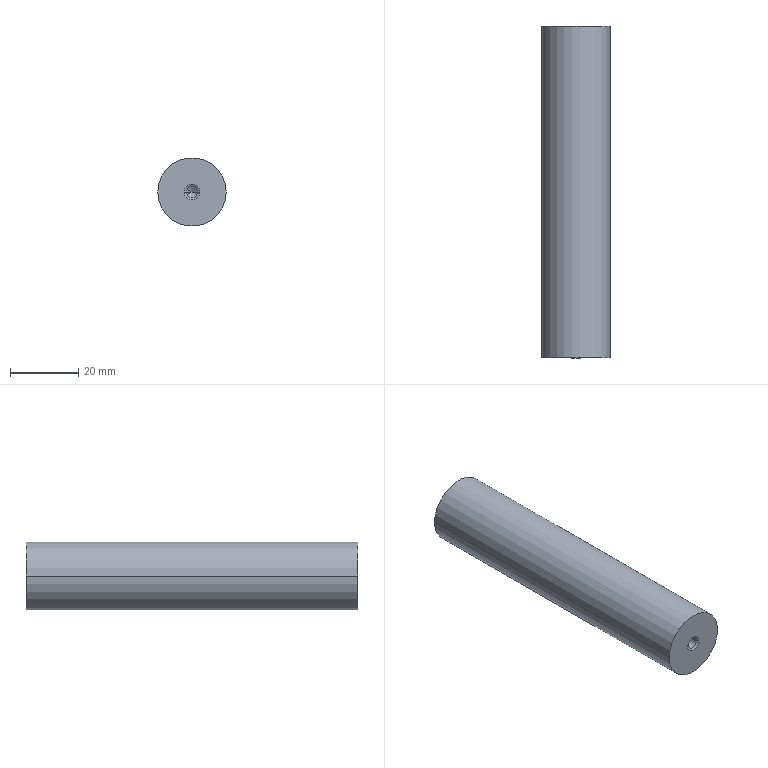Part | NX | 1 solid | 16 faces | box 20 x 97 x 20 mm | volume 30242 mm3 | cone 8 | cylinder 6 | plane 2 | commonest cylinder face diameters 3.3 x4 20 x2
STEP:
#1=CARTESIAN_POINT('',(10.,-28.5,0.));
#2=VERTEX_POINT('',#1);
#3=CARTESIAN_POINT('',(-10.,-28.5,0.));
#4=VERTEX_POINT('',#3);
#5=CARTESIAN_POINT('',(0.,-28.5,0.));
#6=DIRECTION('',(0.,1.,0.));
#7=DIRECTION('',(1.,0.,0.));
#8=AXIS2_PLACEMENT_3D('',#5,#6,#7);
#9=CIRCLE('',#8,10.);
#10=EDGE_CURVE('',#2,#4,#9,.T.);
#11=ORIENTED_EDGE('',*,*,#10,.T.);
#12=CARTESIAN_POINT('',(-10.,68.5,0.));
#13=VERTEX_POINT('',#12);
#14=CARTESIAN_POINT('',(-10.,-44.35,0.));
#15=DIRECTION('',(0.,1.,0.));
#16=VECTOR('',#15,1000.);
#17=LINE('',#14,#16);
#18=EDGE_CURVE('',#13,#4,#17,.F.);
#19=ORIENTED_EDGE('',*,*,#18,.F.);
#20=CARTESIAN_POINT('',(10.,68.5,0.));
#21=VERTEX_POINT('',#20);
#22=CARTESIAN_POINT('',(0.,68.5,0.));
#23=DIRECTION('',(0.,1.,0.));
#24=DIRECTION('',(1.,0.,0.));
#25=AXIS2_PLACEMENT_3D('',#22,#23,#24);
#26=CIRCLE('',#25,10.);
#27=EDGE_CURVE('',#21,#13,#26,.T.);
#28=ORIENTED_EDGE('',*,*,#27,.F.);
#29=CARTESIAN_POINT('',(10.,-44.35,0.));
#30=DIRECTION('',(0.,1.,0.));
#31=VECTOR('',#30,1000.);
#32=LINE('',#29,#31);
#33=EDGE_CURVE('',#21,#2,#32,.F.);
#34=ORIENTED_EDGE('',*,*,#33,.T.);
#35=EDGE_LOOP('',(#11,#19,#28,#34));
#36=FACE_BOUND('',#35,.T.);
#37=CARTESIAN_POINT('',(0.,-44.35,0.));
#38=DIRECTION('',(0.,1.,0.));
#39=DIRECTION('',(1.,0.,0.));
#40=AXIS2_PLACEMENT_3D('',#37,#38,#39);
#41=CYLINDRICAL_SURFACE('',#40,10.);
#42=ADVANCED_FACE('',(#36),#41,.T.);
#43=CARTESIAN_POINT('',(0.,68.5,0.));
#44=DIRECTION('',(0.,1.,0.));
#45=DIRECTION('',(1.,0.,0.));
#46=AXIS2_PLACEMENT_3D('',#43,#44,#45);
#47=CIRCLE('',#46,10.);
#48=EDGE_CURVE('',#13,#21,#47,.T.);
#49=ORIENTED_EDGE('',*,*,#48,.T.);
#50=ORIENTED_EDGE('',*,*,#27,.T.);
#51=EDGE_LOOP('',(#49,#50));
#52=FACE_BOUND('',#51,.T.);
#53=CARTESIAN_POINT('',(-2.315,68.5,0.));
#54=VERTEX_POINT('',#53);
#55=CARTESIAN_POINT('',(2.315,68.5,0.));
#56=VERTEX_POINT('',#55);
#57=CARTESIAN_POINT('',(0.,68.5,0.));
#58=DIRECTION('',(0.,1.,0.));
#59=DIRECTION('',(1.,0.,0.));
#60=AXIS2_PLACEMENT_3D('',#57,#58,#59);
#61=CIRCLE('',#60,2.315);
#62=EDGE_CURVE('',#54,#56,#61,.T.);
#63=ORIENTED_EDGE('',*,*,#62,.F.);
#64=CARTESIAN_POINT('',(0.,68.5,0.));
#65=DIRECTION('',(0.,1.,0.));
#66=DIRECTION('',(1.,0.,0.));
#67=AXIS2_PLACEMENT_3D('',#64,#65,#66);
#68=CIRCLE('',#67,2.315);
#69=EDGE_CURVE('',#56,#54,#68,.T.);
#70=ORIENTED_EDGE('',*,*,#69,.F.);
#71=EDGE_LOOP('',(#63,#70));
#72=FACE_BOUND('',#71,.T.);
#73=CARTESIAN_POINT('',(0.,68.5,0.));
#74=DIRECTION('',(0.,1.,0.));
#75=DIRECTION('',(1.,0.,0.));
#76=AXIS2_PLACEMENT_3D('',#73,#74,#75);
#77=PLANE('',#76);
#78=ADVANCED_FACE('',(#52,#72),#77,.T.);
#79=CARTESIAN_POINT('',(1.65,68.116,0.));
#80=VERTEX_POINT('',#79);
#81=CARTESIAN_POINT('',(-1.65,68.116,0.));
#82=VERTEX_POINT('',#81);
#83=CARTESIAN_POINT('',(0.,68.116,0.));
#84=DIRECTION('',(0.,1.,0.));
#85=DIRECTION('',(1.,0.,0.));
#86=AXIS2_PLACEMENT_3D('',#83,#84,#85);
#87=CIRCLE('',#86,1.65);
#88=EDGE_CURVE('',#80,#82,#87,.T.);
#89=ORIENTED_EDGE('',*,*,#88,.F.);
#90=CARTESIAN_POINT('',(1.65,68.116,0.));
#91=DIRECTION('',(0.866,0.5,0.));
#92=VECTOR('',#91,1000.);
#93=LINE('',#90,#92);
#94=EDGE_CURVE('',#80,#56,#93,.T.);
#95=ORIENTED_EDGE('',*,*,#94,.T.);
#96=ORIENTED_EDGE('',*,*,#69,.T.);
#97=CARTESIAN_POINT('',(-1.65,68.116,0.));
#98=DIRECTION('',(-0.866,0.5,0.));
#99=VECTOR('',#98,1000.);
#100=LINE('',#97,#99);
#101=EDGE_CURVE('',#82,#54,#100,.T.);
#102=ORIENTED_EDGE('',*,*,#101,.F.);
#103=EDGE_LOOP('',(#89,#95,#96,#102));
#104=FACE_BOUND('',#103,.T.);
#105=CARTESIAN_POINT('',(0.,68.116,0.));
#106=DIRECTION('',(0.,1.,0.));
#107=DIRECTION('',(1.,0.,0.));
#108=AXIS2_PLACEMENT_3D('',#105,#106,#107);
#109=CONICAL_SURFACE('',#108,1.65,1.047);
#110=ADVANCED_FACE('',(#104),#109,.F.);
#111=ORIENTED_EDGE('',*,*,#10,.F.);
#112=CARTESIAN_POINT('',(0.,-28.5,0.));
#113=DIRECTION('',(0.,1.,0.));
#114=DIRECTION('',(1.,0.,0.));
#115=AXIS2_PLACEMENT_3D('',#112,#113,#114);
#116=CIRCLE('',#115,10.);
#117=EDGE_CURVE('',#4,#2,#116,.T.);
#118=ORIENTED_EDGE('',*,*,#117,.F.);
#119=EDGE_LOOP('',(#111,#118));
#120=FACE_BOUND('',#119,.T.);
#121=CARTESIAN_POINT('',(-2.315,-28.5,0.));
#122=VERTEX_POINT('',#121);
#123=CARTESIAN_POINT('',(2.315,-28.5,0.));
#124=VERTEX_POINT('',#123);
#125=CARTESIAN_POINT('',(0.,-28.5,0.));
#126=DIRECTION('',(0.,-1.,0.));
#127=DIRECTION('',(-1.,0.,0.));
#128=AXIS2_PLACEMENT_3D('',#125,#126,#127);
#129=CIRCLE('',#128,2.315);
#130=EDGE_CURVE('',#122,#124,#129,.T.);
#131=ORIENTED_EDGE('',*,*,#130,.F.);
#132=CARTESIAN_POINT('',(0.,-28.5,0.));
#133=DIRECTION('',(0.,-1.,0.));
#134=DIRECTION('',(-1.,0.,0.));
#135=AXIS2_PLACEMENT_3D('',#132,#133,#134);
#136=CIRCLE('',#135,2.315);
#137=EDGE_CURVE('',#124,#122,#136,.T.);
#138=ORIENTED_EDGE('',*,*,#137,.F.);
#139=EDGE_LOOP('',(#131,#138));
#140=FACE_BOUND('',#139,.T.);
#141=CARTESIAN_POINT('',(0.,-28.5,0.));
#142=DIRECTION('',(0.,1.,0.));
#143=DIRECTION('',(1.,0.,0.));
#144=AXIS2_PLACEMENT_3D('',#141,#142,#143);
#145=PLANE('',#144);
#146=ADVANCED_FACE('',(#120,#140),#145,.F.);
#147=CARTESIAN_POINT('',(1.65,-15.5,0.));
#148=VERTEX_POINT('',#147);
#149=CARTESIAN_POINT('',(-1.65,-15.5,0.));
#150=VERTEX_POINT('',#149);
#151=CARTESIAN_POINT('',(0.,-15.5,0.));
#152=DIRECTION('',(0.,-1.,0.));
#153=DIRECTION('',(-1.,0.,0.));
#154=AXIS2_PLACEMENT_3D('',#151,#152,#153);
#155=CIRCLE('',#154,1.65);
#156=EDGE_CURVE('',#148,#150,#155,.T.);
#157=ORIENTED_EDGE('',*,*,#156,.F.);
#158=CARTESIAN_POINT('',(1.65,-28.116,0.));
#159=VERTEX_POINT('',#158);
#160=CARTESIAN_POINT('',(1.65,-38.5,0.));
#161=DIRECTION('',(0.,-1.,0.));
#162=VECTOR('',#161,1000.);
#163=LINE('',#160,#162);
#164=EDGE_CURVE('',#159,#148,#163,.F.);
#165=ORIENTED_EDGE('',*,*,#164,.F.);
#166=CARTESIAN_POINT('',(-1.65,-28.116,0.));
#167=VERTEX_POINT('',#166);
#168=CARTESIAN_POINT('',(0.,-28.116,0.));
#169=DIRECTION('',(0.,-1.,0.));
#170=DIRECTION('',(-1.,0.,0.));
#171=AXIS2_PLACEMENT_3D('',#168,#169,#170);
#172=CIRCLE('',#171,1.65);
#173=EDGE_CURVE('',#159,#167,#172,.T.);
#174=ORIENTED_EDGE('',*,*,#173,.T.);
#175=CARTESIAN_POINT('',(-1.65,-38.5,0.));
#176=DIRECTION('',(0.,-1.,0.));
#177=VECTOR('',#176,1000.);
#178=LINE('',#175,#177);
#179=EDGE_CURVE('',#167,#150,#178,.F.);
#180=ORIENTED_EDGE('',*,*,#179,.T.);
#181=EDGE_LOOP('',(#157,#165,#174,#180));
#182=FACE_BOUND('',#181,.T.);
#183=CARTESIAN_POINT('',(0.,-38.5,0.));
#184=DIRECTION('',(0.,-1.,0.));
#185=DIRECTION('',(-1.,0.,0.));
#186=AXIS2_PLACEMENT_3D('',#183,#184,#185);
#187=CYLINDRICAL_SURFACE('',#186,1.65);
#188=ADVANCED_FACE('',(#182),#187,.F.);
#189=ORIENTED_EDGE('',*,*,#156,.T.);
#190=CARTESIAN_POINT('',(0.,-14.509,0.));
#191=VERTEX_POINT('',#190);
#192=CARTESIAN_POINT('',(-1.65,-15.5,0.));
#193=DIRECTION('',(-0.8572,-0.515,0.));
#194=VECTOR('',#193,1000.);
#195=LINE('',#192,#194);
#196=EDGE_CURVE('',#191,#150,#195,.T.);
#197=ORIENTED_EDGE('',*,*,#196,.F.);
#198=CARTESIAN_POINT('',(1.65,-15.5,0.));
#199=DIRECTION('',(0.8572,-0.515,0.));
#200=VECTOR('',#199,1000.);
#201=LINE('',#198,#200);
#202=EDGE_CURVE('',#191,#148,#201,.T.);
#203=ORIENTED_EDGE('',*,*,#202,.T.);
#204=EDGE_LOOP('',(#189,#197,#203));
#205=FACE_BOUND('',#204,.T.);
#206=CARTESIAN_POINT('',(0.,-15.5,0.));
#207=DIRECTION('',(0.,-1.,0.));
#208=DIRECTION('',(-1.,0.,0.));
#209=AXIS2_PLACEMENT_3D('',#206,#207,#208);
#210=CONICAL_SURFACE('',#209,1.65,1.03);
#211=ADVANCED_FACE('',(#205),#210,.F.);
#212=CARTESIAN_POINT('',(1.65,55.5,0.));
#213=VERTEX_POINT('',#212);
#214=CARTESIAN_POINT('',(-1.65,55.5,0.));
#215=VERTEX_POINT('',#214);
#216=CARTESIAN_POINT('',(0.,55.5,0.));
#217=DIRECTION('',(0.,1.,0.));
#218=DIRECTION('',(1.,0.,0.));
#219=AXIS2_PLACEMENT_3D('',#216,#217,#218);
#220=CIRCLE('',#219,1.65);
#221=EDGE_CURVE('',#213,#215,#220,.T.);
#222=ORIENTED_EDGE('',*,*,#221,.T.);
#223=CARTESIAN_POINT('',(0.,54.509,0.));
#224=VERTEX_POINT('',#223);
#225=CARTESIAN_POINT('',(-1.65,55.5,0.));
#226=DIRECTION('',(-0.8572,0.515,0.));
#227=VECTOR('',#226,1000.);
#228=LINE('',#225,#227);
#229=EDGE_CURVE('',#215,#224,#228,.F.);
#230=ORIENTED_EDGE('',*,*,#229,.T.);
#231=CARTESIAN_POINT('',(1.65,55.5,0.));
#232=DIRECTION('',(0.8572,0.515,0.));
#233=VECTOR('',#232,1000.);
#234=LINE('',#231,#233);
#235=EDGE_CURVE('',#213,#224,#234,.F.);
#236=ORIENTED_EDGE('',*,*,#235,.F.);
#237=EDGE_LOOP('',(#222,#230,#236));
#238=FACE_BOUND('',#237,.T.);
#239=CARTESIAN_POINT('',(0.,55.5,0.));
#240=DIRECTION('',(0.,1.,0.));
#241=DIRECTION('',(1.,0.,0.));
#242=AXIS2_PLACEMENT_3D('',#239,#240,#241);
#243=CONICAL_SURFACE('',#242,1.65,1.03);
#244=ADVANCED_FACE('',(#238),#243,.F.);
#245=ORIENTED_EDGE('',*,*,#221,.F.);
#246=CARTESIAN_POINT('',(1.65,78.5,0.));
#247=DIRECTION('',(0.,1.,0.));
#248=VECTOR('',#247,1000.);
#249=LINE('',#246,#248);
#250=EDGE_CURVE('',#213,#80,#249,.T.);
#251=ORIENTED_EDGE('',*,*,#250,.T.);
#252=ORIENTED_EDGE('',*,*,#88,.T.);
#253=CARTESIAN_POINT('',(-1.65,78.5,0.));
#254=DIRECTION('',(0.,1.,0.));
#255=VECTOR('',#254,1000.);
#256=LINE('',#253,#255);
#257=EDGE_CURVE('',#215,#82,#256,.T.);
#258=ORIENTED_EDGE('',*,*,#257,.F.);
#259=EDGE_LOOP('',(#245,#251,#252,#258));
#260=FACE_BOUND('',#259,.T.);
#261=CARTESIAN_POINT('',(0.,78.5,0.));
#262=DIRECTION('',(0.,1.,0.));
#263=DIRECTION('',(1.,0.,0.));
#264=AXIS2_PLACEMENT_3D('',#261,#262,#263);
#265=CYLINDRICAL_SURFACE('',#264,1.65);
#266=ADVANCED_FACE('',(#260),#265,.F.);
#267=ORIENTED_EDGE('',*,*,#130,.T.);
#268=CARTESIAN_POINT('',(1.65,-28.116,0.));
#269=DIRECTION('',(0.866,-0.5,0.));
#270=VECTOR('',#269,1000.);
#271=LINE('',#268,#270);
#272=EDGE_CURVE('',#159,#124,#271,.T.);
#273=ORIENTED_EDGE('',*,*,#272,.F.);
#274=CARTESIAN_POINT('',(0.,-28.116,0.));
#275=DIRECTION('',(0.,-1.,0.));
#276=DIRECTION('',(-1.,0.,0.));
#277=AXIS2_PLACEMENT_3D('',#274,#275,#276);
#278=CIRCLE('',#277,1.65);
#279=EDGE_CURVE('',#167,#159,#278,.T.);
#280=ORIENTED_EDGE('',*,*,#279,.F.);
#281=CARTESIAN_POINT('',(-1.65,-28.116,0.));
#282=DIRECTION('',(-0.866,-0.5,0.));
#283=VECTOR('',#282,1000.);
#284=LINE('',#281,#283);
#285=EDGE_CURVE('',#167,#122,#284,.T.);
#286=ORIENTED_EDGE('',*,*,#285,.T.);
#287=EDGE_LOOP('',(#267,#273,#280,#286));
#288=FACE_BOUND('',#287,.T.);
#289=CARTESIAN_POINT('',(0.,-28.116,0.));
#290=DIRECTION('',(0.,-1.,0.));
#291=DIRECTION('',(-1.,0.,0.));
#292=AXIS2_PLACEMENT_3D('',#289,#290,#291);
#293=CONICAL_SURFACE('',#292,1.65,1.047);
#294=ADVANCED_FACE('',(#288),#293,.F.);
#295=ORIENTED_EDGE('',*,*,#202,.F.);
#296=ORIENTED_EDGE('',*,*,#196,.T.);
#297=CARTESIAN_POINT('',(0.,-15.5,0.));
#298=DIRECTION('',(0.,-1.,0.));
#299=DIRECTION('',(-1.,0.,0.));
#300=AXIS2_PLACEMENT_3D('',#297,#298,#299);
#301=CIRCLE('',#300,1.65);
#302=EDGE_CURVE('',#150,#148,#301,.T.);
#303=ORIENTED_EDGE('',*,*,#302,.T.);
#304=EDGE_LOOP('',(#295,#296,#303));
#305=FACE_BOUND('',#304,.T.);
#306=CARTESIAN_POINT('',(0.,-15.5,0.));
#307=DIRECTION('',(0.,-1.,0.));
#308=DIRECTION('',(-1.,0.,0.));
#309=AXIS2_PLACEMENT_3D('',#306,#307,#308);
#310=CONICAL_SURFACE('',#309,1.65,1.03);
#311=ADVANCED_FACE('',(#305),#310,.F.);
#312=ORIENTED_EDGE('',*,*,#179,.F.);
#313=ORIENTED_EDGE('',*,*,#279,.T.);
#314=ORIENTED_EDGE('',*,*,#164,.T.);
#315=ORIENTED_EDGE('',*,*,#302,.F.);
#316=EDGE_LOOP('',(#312,#313,#314,#315));
#317=FACE_BOUND('',#316,.T.);
#318=CARTESIAN_POINT('',(0.,-38.5,0.));
#319=DIRECTION('',(0.,-1.,0.));
#320=DIRECTION('',(-1.,0.,0.));
#321=AXIS2_PLACEMENT_3D('',#318,#319,#320);
#322=CYLINDRICAL_SURFACE('',#321,1.65);
#323=ADVANCED_FACE('',(#317),#322,.F.);
#324=ORIENTED_EDGE('',*,*,#173,.F.);
#325=ORIENTED_EDGE('',*,*,#272,.T.);
#326=ORIENTED_EDGE('',*,*,#137,.T.);
#327=ORIENTED_EDGE('',*,*,#285,.F.);
#328=EDGE_LOOP('',(#324,#325,#326,#327));
#329=FACE_BOUND('',#328,.T.);
#330=CARTESIAN_POINT('',(0.,-28.116,0.));
#331=DIRECTION('',(0.,-1.,0.));
#332=DIRECTION('',(-1.,0.,0.));
#333=AXIS2_PLACEMENT_3D('',#330,#331,#332);
#334=CONICAL_SURFACE('',#333,1.65,1.047);
#335=ADVANCED_FACE('',(#329),#334,.F.);
#336=ORIENTED_EDGE('',*,*,#229,.F.);
#337=CARTESIAN_POINT('',(0.,55.5,0.));
#338=DIRECTION('',(0.,1.,0.));
#339=DIRECTION('',(1.,0.,0.));
#340=AXIS2_PLACEMENT_3D('',#337,#338,#339);
#341=CIRCLE('',#340,1.65);
#342=EDGE_CURVE('',#215,#213,#341,.T.);
#343=ORIENTED_EDGE('',*,*,#342,.T.);
#344=ORIENTED_EDGE('',*,*,#235,.T.);
#345=EDGE_LOOP('',(#336,#343,#344));
#346=FACE_BOUND('',#345,.T.);
#347=CARTESIAN_POINT('',(0.,55.5,0.));
#348=DIRECTION('',(0.,1.,0.));
#349=DIRECTION('',(1.,0.,0.));
#350=AXIS2_PLACEMENT_3D('',#347,#348,#349);
#351=CONICAL_SURFACE('',#350,1.65,1.03);
#352=ADVANCED_FACE('',(#346),#351,.F.);
#353=ORIENTED_EDGE('',*,*,#250,.F.);
#354=ORIENTED_EDGE('',*,*,#342,.F.);
#355=ORIENTED_EDGE('',*,*,#257,.T.);
#356=CARTESIAN_POINT('',(0.,68.116,0.));
#357=DIRECTION('',(0.,1.,0.));
#358=DIRECTION('',(1.,0.,0.));
#359=AXIS2_PLACEMENT_3D('',#356,#357,#358);
#360=CIRCLE('',#359,1.65);
#361=EDGE_CURVE('',#82,#80,#360,.T.);
#362=ORIENTED_EDGE('',*,*,#361,.T.);
#363=EDGE_LOOP('',(#353,#354,#355,#362));
#364=FACE_BOUND('',#363,.T.);
#365=CARTESIAN_POINT('',(0.,78.5,0.));
#366=DIRECTION('',(0.,1.,0.));
#367=DIRECTION('',(1.,0.,0.));
#368=AXIS2_PLACEMENT_3D('',#365,#366,#367);
#369=CYLINDRICAL_SURFACE('',#368,1.65);
#370=ADVANCED_FACE('',(#364),#369,.F.);
#371=ORIENTED_EDGE('',*,*,#48,.F.);
#372=ORIENTED_EDGE('',*,*,#18,.T.);
#373=ORIENTED_EDGE('',*,*,#117,.T.);
#374=ORIENTED_EDGE('',*,*,#33,.F.);
#375=EDGE_LOOP('',(#371,#372,#373,#374));
#376=FACE_BOUND('',#375,.T.);
#377=CARTESIAN_POINT('',(0.,-44.35,0.));
#378=DIRECTION('',(0.,1.,0.));
#379=DIRECTION('',(1.,0.,0.));
#380=AXIS2_PLACEMENT_3D('',#377,#378,#379);
#381=CYLINDRICAL_SURFACE('',#380,10.);
#382=ADVANCED_FACE('',(#376),#381,.T.);
#383=ORIENTED_EDGE('',*,*,#62,.T.);
#384=ORIENTED_EDGE('',*,*,#94,.F.);
#385=ORIENTED_EDGE('',*,*,#361,.F.);
#386=ORIENTED_EDGE('',*,*,#101,.T.);
#387=EDGE_LOOP('',(#383,#384,#385,#386));
#388=FACE_BOUND('',#387,.T.);
#389=CARTESIAN_POINT('',(0.,68.116,0.));
#390=DIRECTION('',(0.,1.,0.));
#391=DIRECTION('',(1.,0.,0.));
#392=AXIS2_PLACEMENT_3D('',#389,#390,#391);
#393=CONICAL_SURFACE('',#392,1.65,1.047);
#394=ADVANCED_FACE('',(#388),#393,.F.);
#395=CLOSED_SHELL('',(#42,#78,#110,#146,#188,#211,#244,#266,#294,#311,#323,#335,#352,#370,#382,#394));
#396=MANIFOLD_SOLID_BREP('',#395);
#397=(LENGTH_UNIT()NAMED_UNIT(*)SI_UNIT(.MILLI.,.METRE.));
#398=UNCERTAINTY_MEASURE_WITH_UNIT(LENGTH_MEASURE(0.00001),#397,'','');
#399=(NAMED_UNIT(*)PLANE_ANGLE_UNIT()SI_UNIT($,.RADIAN.));
#400=(NAMED_UNIT(*)SI_UNIT($,.STERADIAN.)SOLID_ANGLE_UNIT());
#401=(GEOMETRIC_REPRESENTATION_CONTEXT(3)GLOBAL_UNCERTAINTY_ASSIGNED_CONTEXT((#398))GLOBAL_UNIT_ASSIGNED_CONTEXT((#397,#399,#400))REPRESENTATION_CONTEXT('',''));
#402=ADVANCED_BREP_SHAPE_REPRESENTATION('',(#396),#401);